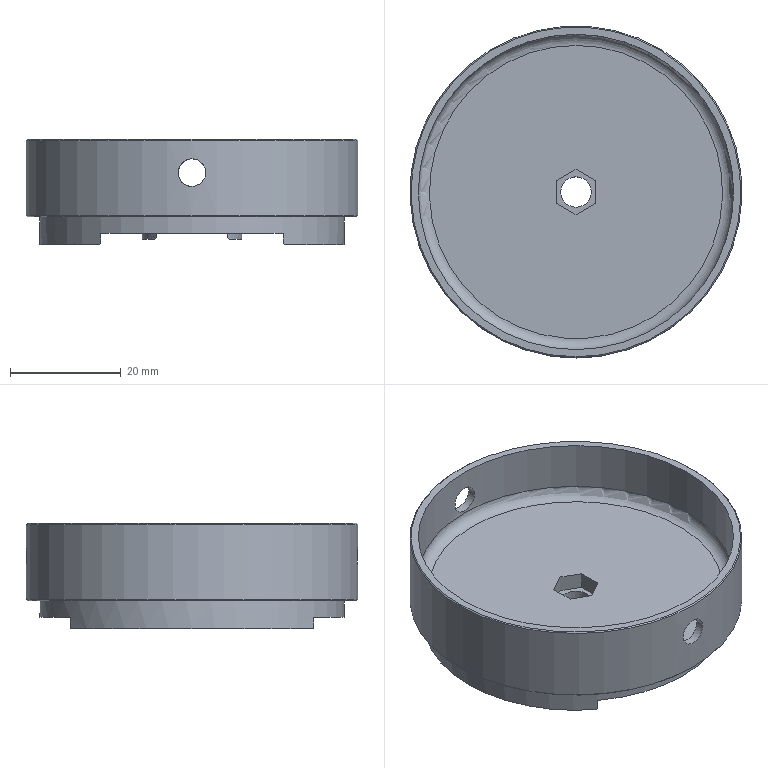NC program | NX | posted with a generic post | part box 60 x 60 x 19 mm
Lines 2835 to 4306 of 4306:
(FLOOR_WALL_1 , TOOL : D6)
N5644 T07 M6
N5646 G54
N5648 G17 G0 G90 X-2.875 Y34.477 S4500 M3
N5650 G43 Z30. H7
N5652 Z1.4
N5654 G94 G1 Z-0.1 F1000.
N5656 X-0.52 Y30.397
N5658 G3 X0. Y30.097 R0.6
N5660 G2 X16.243 Y25.337 R30.097 F1800.
N5662 G1 X13.4 Y23.916
N5664 Y-23.916
N5666 X16.243 Y-25.337
N5668 G2 X-16.243 Y-25.337 R30.097
N5670 G1 X-13.4 Y-23.916
N5672 Y23.916
N5674 X-16.243 Y25.337
N5676 G2 X0. Y30.097 R30.097
N5678 G1 Y25.897
N5680 G2 X9.21 Y24.204 R25.897
N5682 G3 X9.2 Y23.916 R4.2
N5684 G1 Y-23.916
N5686 G3 X9.21 Y-24.204 R4.2
N5688 G2 X-9.21 Y-24.204 R25.897
N5690 G3 X-9.2 Y-23.916 R4.2
N5692 G1 Y23.916
N5694 G3 X-9.21 Y24.204 R4.2
N5696 G2 X0. Y25.897 R25.897
N5698 G1 Y21.697
N5700 G2 X5. Y21.113 R21.697
N5702 G1 Y-21.113
N5704 G2 X-5. Y-21.113 R21.697
N5706 G1 Y21.113
N5708 G2 X0. Y21.697 R21.697
N5710 G1 Y17.497
N5712 G2 X0.8 Y17.479 R17.497
N5714 G1 Y-17.479
N5716 G2 X-0.8 Y-17.479 R17.497
N5718 G1 Y17.479
N5720 G2 X0. Y17.497 R17.497
N5722 G3 X0.52 Y17.797 R0.6
N5724 G1 Z1.4
N5726 G0 X-2.875 Y34.477 Z1.3
N5728 G1 Z-0.2 F1000.
N5730 X-0.52 Y30.397
N5732 G3 X0. Y30.097 R0.6
N5734 G2 X16.243 Y25.337 R30.097 F1800.
N5736 G1 X13.4 Y23.916
N5738 Y-23.916
N5740 X16.243 Y-25.337
N5742 G2 X-16.243 Y-25.337 R30.097
N5744 G1 X-13.4 Y-23.916
N5746 Y23.916
N5748 X-16.243 Y25.337
N5750 G2 X0. Y30.097 R30.097
N5752 G1 Y25.897
N5754 G2 X9.21 Y24.204 R25.897
N5756 G3 X9.2 Y23.916 R4.2
N5758 G1 Y-23.916
N5760 G3 X9.21 Y-24.204 R4.2
N5762 G2 X-9.21 Y-24.204 R25.897
N5764 G3 X-9.2 Y-23.916 R4.2
N5766 G1 Y23.916
N5768 G3 X-9.21 Y24.204 R4.2
N5770 G2 X0. Y25.897 R25.897
N5772 G1 Y21.697
N5774 G2 X5. Y21.113 R21.697
N5776 G1 Y-21.113
N5778 G2 X-5. Y-21.113 R21.697
N5780 G1 Y21.113
N5782 G2 X0. Y21.697 R21.697
N5784 G1 Y17.497
N5786 G2 X0.8 Y17.479 R17.497
N5788 G1 Y-17.479
N5790 G2 X-0.8 Y-17.479 R17.497
N5792 G1 Y17.479
N5794 G2 X0. Y17.497 R17.497
N5796 G3 X0.52 Y17.797 R0.6
N5798 G1 Z1.3
N5800 G0 X-2.875 Y34.477 Z1.2
N5802 G1 Z-0.3 F1000.
N5804 X-0.52 Y30.397
N5806 G3 X0. Y30.097 R0.6
N5808 G2 X16.243 Y25.337 R30.097 F1800.
N5810 G1 X13.4 Y23.916
N5812 Y-23.916
N5814 X16.243 Y-25.337
N5816 G2 X-16.243 Y-25.337 R30.097
N5818 G1 X-13.4 Y-23.916
N5820 Y23.916
N5822 X-16.243 Y25.337
N5824 G2 X0. Y30.097 R30.097
N5826 G1 Y25.897
N5828 G2 X9.21 Y24.204 R25.897
N5830 G3 X9.2 Y23.916 R4.2
N5832 G1 Y-23.916
N5834 G3 X9.21 Y-24.204 R4.2
N5836 G2 X-9.21 Y-24.204 R25.897
N5838 G3 X-9.2 Y-23.916 R4.2
N5840 G1 Y23.916
N5842 G3 X-9.21 Y24.204 R4.2
N5844 G2 X0. Y25.897 R25.897
N5846 G1 Y21.697
N5848 G2 X5. Y21.113 R21.697
N5850 G1 Y-21.113
N5852 G2 X-5. Y-21.113 R21.697
N5854 G1 Y21.113
N5856 G2 X0. Y21.697 R21.697
N5858 G1 Y17.497
N5860 G2 X0.8 Y17.479 R17.497
N5862 G1 Y-17.479
N5864 G2 X-0.8 Y-17.479 R17.497
N5866 G1 Y17.479
N5868 G2 X0. Y17.497 R17.497
N5870 G3 X0.52 Y17.797 R0.6
N5872 G1 Z1.2
N5874 G0 X-2.875 Y34.477 Z1.1
N5876 G1 Z-0.4 F1000.
N5878 X-0.52 Y30.397
N5880 G3 X0. Y30.097 R0.6
N5882 G2 X16.243 Y25.337 R30.097 F1800.
N5884 G1 X13.4 Y23.916
N5886 Y-23.916
N5888 X16.243 Y-25.337
N5890 G2 X-16.243 Y-25.337 R30.097
N5892 G1 X-13.4 Y-23.916
N5894 Y23.916
N5896 X-16.243 Y25.337
N5898 G2 X0. Y30.097 R30.097
N5900 G1 Y25.897
N5902 G2 X9.21 Y24.204 R25.897
N5904 G3 X9.2 Y23.916 R4.2
N5906 G1 Y-23.916
N5908 G3 X9.21 Y-24.204 R4.2
N5910 G2 X-9.21 Y-24.204 R25.897
N5912 G3 X-9.2 Y-23.916 R4.2
N5914 G1 Y23.916
N5916 G3 X-9.21 Y24.204 R4.2
N5918 G2 X0. Y25.897 R25.897
N5920 G1 Y21.697
N5922 G2 X5. Y21.113 R21.697
N5924 G1 Y-21.113
N5926 G2 X-5. Y-21.113 R21.697
N5928 G1 Y21.113
N5930 G2 X0. Y21.697 R21.697
N5932 G1 Y17.497
N5934 G2 X0.8 Y17.479 R17.497
N5936 G1 Y-17.479
N5938 G2 X-0.8 Y-17.479 R17.497
N5940 G1 Y17.479
N5942 G2 X0. Y17.497 R17.497
N5944 G3 X0.52 Y17.797 R0.6
N5946 G1 Z1.1
N5948 G0 X-2.875 Y34.477 Z1.
N5950 G1 Z-0.5 F1000.
N5952 X-0.52 Y30.397
N5954 G3 X0. Y30.097 R0.6
N5956 G2 X16.243 Y25.337 R30.097 F1800.
N5958 G1 X13.4 Y23.916
N5960 Y-23.916
N5962 X16.243 Y-25.337
N5964 G2 X-16.243 Y-25.337 R30.097
N5966 G1 X-13.4 Y-23.916
N5968 Y23.916
N5970 X-16.243 Y25.337
N5972 G2 X0. Y30.097 R30.097
N5974 G1 Y25.897
N5976 G2 X9.21 Y24.204 R25.897
N5978 G3 X9.2 Y23.916 R4.2
N5980 G1 Y-23.916
N5982 G3 X9.21 Y-24.204 R4.2
N5984 G2 X-9.21 Y-24.204 R25.897
N5986 G3 X-9.2 Y-23.916 R4.2
N5988 G1 Y23.916
N5990 G3 X-9.21 Y24.204 R4.2
N5992 G2 X0. Y25.897 R25.897
N5994 G1 Y21.697
N5996 G2 X5. Y21.113 R21.697
N5998 G1 Y-21.113
N6000 G2 X-5. Y-21.113 R21.697
N6002 G1 Y21.113
N6004 G2 X0. Y21.697 R21.697
N6006 G1 Y17.497
N6008 G2 X0.8 Y17.479 R17.497
N6010 G1 Y-17.479
N6012 G2 X-0.8 Y-17.479 R17.497
N6014 G1 Y17.479
N6016 G2 X0. Y17.497 R17.497
N6018 G3 X0.52 Y17.797 R0.6
N6020 G1 Z1.
N6022 G0 X-2.875 Y34.477 Z0.9
N6024 G1 Z-0.6 F1000.
N6026 X-0.52 Y30.397
N6028 G3 X0. Y30.097 R0.6
N6030 G2 X16.243 Y25.337 R30.097 F1800.
N6032 G1 X13.4 Y23.916
N6034 Y-23.916
N6036 X16.243 Y-25.337
N6038 G2 X-16.243 Y-25.337 R30.097
N6040 G1 X-13.4 Y-23.916
N6042 Y23.916
N6044 X-16.243 Y25.337
N6046 G2 X0. Y30.097 R30.097
N6048 G1 Y25.897
N6050 G2 X9.21 Y24.204 R25.897
N6052 G3 X9.2 Y23.916 R4.2
N6054 G1 Y-23.916
N6056 G3 X9.21 Y-24.204 R4.2
N6058 G2 X-9.21 Y-24.204 R25.897
N6060 G3 X-9.2 Y-23.916 R4.2
N6062 G1 Y23.916
N6064 G3 X-9.21 Y24.204 R4.2
N6066 G2 X0. Y25.897 R25.897
N6068 G1 Y21.697
N6070 G2 X5. Y21.113 R21.697
N6072 G1 Y-21.113
N6074 G2 X-5. Y-21.113 R21.697
N6076 G1 Y21.113
N6078 G2 X0. Y21.697 R21.697
N6080 G1 Y17.497
N6082 G2 X0.8 Y17.479 R17.497
N6084 G1 Y-17.479
N6086 G2 X-0.8 Y-17.479 R17.497
N6088 G1 Y17.479
N6090 G2 X0. Y17.497 R17.497
N6092 G3 X0.52 Y17.797 R0.6
N6094 G1 Z0.9
N6096 G0 X-2.875 Y34.477 Z0.8
N6098 G1 Z-0.7 F1000.
N6100 X-0.52 Y30.397
N6102 G3 X0. Y30.097 R0.6
N6104 G2 X16.243 Y25.337 R30.097 F1800.
N6106 G1 X13.4 Y23.916
N6108 Y-23.916
N6110 X16.243 Y-25.337
N6112 G2 X-16.243 Y-25.337 R30.097
N6114 G1 X-13.4 Y-23.916
N6116 Y23.916
N6118 X-16.243 Y25.337
N6120 G2 X0. Y30.097 R30.097
N6122 G1 Y25.897
N6124 G2 X9.21 Y24.204 R25.897
N6126 G3 X9.2 Y23.916 R4.2
N6128 G1 Y-23.916
N6130 G3 X9.21 Y-24.204 R4.2
N6132 G2 X-9.21 Y-24.204 R25.897
N6134 G3 X-9.2 Y-23.916 R4.2
N6136 G1 Y23.916
N6138 G3 X-9.21 Y24.204 R4.2
N6140 G2 X0. Y25.897 R25.897
N6142 G1 Y21.697
N6144 G2 X5. Y21.113 R21.697
N6146 G1 Y-21.113
N6148 G2 X-5. Y-21.113 R21.697
N6150 G1 Y21.113
N6152 G2 X0. Y21.697 R21.697
N6154 G1 Y17.497
N6156 G2 X0.8 Y17.479 R17.497
N6158 G1 Y-17.479
N6160 G2 X-0.8 Y-17.479 R17.497
N6162 G1 Y17.479
N6164 G2 X0. Y17.497 R17.497
N6166 G3 X0.52 Y17.797 R0.6
N6168 G1 Z0.8
N6170 G0 X-2.875 Y34.477 Z0.7
N6172 G1 Z-0.8 F1000.
N6174 X-0.52 Y30.397
N6176 G3 X0. Y30.097 R0.6
N6178 G2 X16.243 Y25.337 R30.097 F1800.
N6180 G1 X13.4 Y23.916
N6182 Y-23.916
N6184 X16.243 Y-25.337
N6186 G2 X-16.243 Y-25.337 R30.097
N6188 G1 X-13.4 Y-23.916
N6190 Y23.916
N6192 X-16.243 Y25.337
N6194 G2 X0. Y30.097 R30.097
N6196 G1 Y25.897
N6198 G2 X9.21 Y24.204 R25.897
N6200 G3 X9.2 Y23.916 R4.2
N6202 G1 Y-23.916
N6204 G3 X9.21 Y-24.204 R4.2
N6206 G2 X-9.21 Y-24.204 R25.897
N6208 G3 X-9.2 Y-23.916 R4.2
N6210 G1 Y23.916
N6212 G3 X-9.21 Y24.204 R4.2
N6214 G2 X0. Y25.897 R25.897
N6216 G1 Y21.697
N6218 G2 X5. Y21.113 R21.697
N6220 G1 Y-21.113
N6222 G2 X-5. Y-21.113 R21.697
N6224 G1 Y21.113
N6226 G2 X0. Y21.697 R21.697
N6228 G1 Y17.497
N6230 G2 X0.8 Y17.479 R17.497
N6232 G1 Y-17.479
N6234 G2 X-0.8 Y-17.479 R17.497
N6236 G1 Y17.479
N6238 G2 X0. Y17.497 R17.497
N6240 G3 X0.52 Y17.797 R0.6
N6242 G1 Z0.7
N6244 G0 X-2.875 Y34.477 Z0.6
N6246 G1 Z-0.9 F1000.
N6248 X-0.52 Y30.397
N6250 G3 X0. Y30.097 R0.6
N6252 G2 X16.243 Y25.337 R30.097 F1800.
N6254 G1 X13.4 Y23.916
N6256 Y-23.916
N6258 X16.243 Y-25.337
N6260 G2 X-16.243 Y-25.337 R30.097
N6262 G1 X-13.4 Y-23.916
N6264 Y23.916
N6266 X-16.243 Y25.337
N6268 G2 X0. Y30.097 R30.097
N6270 G1 Y25.897
N6272 G2 X9.21 Y24.204 R25.897
N6274 G3 X9.2 Y23.916 R4.2
N6276 G1 Y-23.916
N6278 G3 X9.21 Y-24.204 R4.2
N6280 G2 X-9.21 Y-24.204 R25.897
N6282 G3 X-9.2 Y-23.916 R4.2
N6284 G1 Y23.916
N6286 G3 X-9.21 Y24.204 R4.2
N6288 G2 X0. Y25.897 R25.897
N6290 G1 Y21.697
N6292 G2 X5. Y21.113 R21.697
N6294 G1 Y-21.113
N6296 G2 X-5. Y-21.113 R21.697
N6298 G1 Y21.113
N6300 G2 X0. Y21.697 R21.697
N6302 G1 Y17.497
N6304 G2 X0.8 Y17.479 R17.497
N6306 G1 Y-17.479
N6308 G2 X-0.8 Y-17.479 R17.497
N6310 G1 Y17.479
N6312 G2 X0. Y17.497 R17.497
N6314 G3 X0.52 Y17.797 R0.6
N6316 G1 Z0.6
N6318 G0 Z30.
N6320 X-2.875 Y34.477
N6322 Z0.4
N6324 G1 Z-1.1 F1000.
N6326 X-0.52 Y30.397
N6328 G3 X0. Y30.097 R0.6
N6330 G2 X16.243 Y25.337 R30.097 F1800.
N6332 G1 X13.4 Y23.916
N6334 Y-23.916
N6336 X16.243 Y-25.337
N6338 G2 X-16.243 Y-25.337 R30.097
N6340 G1 X-13.4 Y-23.916
N6342 Y23.916
N6344 X-16.243 Y25.337
N6346 G2 X0. Y30.097 R30.097
N6348 G1 Y25.897
N6350 G2 X9.21 Y24.204 R25.897
N6352 G3 X9.2 Y23.916 R4.2
N6354 G1 Y9.102
N6356 X7.896 Y10.464
N6358 G3 X6.976 Y10.662 R0.84
N6360 G1 X3.087 Y9.1
N6362 G3 X2.56 Y8.321 R0.84
N6364 G1 Y-8.321
N6366 G3 X3.087 Y-9.1 R0.84
N6368 G1 X6.976 Y-10.662
N6370 G3 X7.896 Y-10.464 R0.84
N6372 G1 X9.2 Y-9.102
N6374 X8.593 Y-8.521
N6376 X7.289 Y-9.883
N6378 X3.4 Y-8.321
N6380 Y8.321
N6382 X7.289 Y9.883
N6384 X8.739 Y8.369
N6386 G2 X8.739 Y-8.369 R12.1
N6388 G1 X8.593 Y-8.521
N6390 X9.2 Y-9.102
N6392 Y-23.916
N6394 G3 X9.21 Y-24.204 R4.2
N6396 G2 X-9.21 Y-24.204 R25.897
N6398 G3 X-9.2 Y-23.916 R4.2
N6400 G1 Y-9.102
N6402 X-7.896 Y-10.464
N6404 G3 X-6.976 Y-10.662 R0.84
N6406 G1 X-3.087 Y-9.1
N6408 G3 X-2.833 Y-8.941 R0.84
N6410 G1 X0. Y-12.041
N6412 G3 X1.565 Y-13.015 R5.04
N6414 G1 X5. Y-14.394
N6416 Y-21.113
N6418 G2 X-5. Y-21.113 R21.697
N6420 G1 Y-14.394
N6422 X-1.522 Y-12.998
N6424 G3 X0. Y-12.041 R5.04
N6426 G1 Y-16.912
N6428 X0.8 Y-17.234
N6430 Y-17.479
N6432 G2 X-0.8 Y-17.479 R17.497
N6434 G1 Y-17.234
N6436 X0. Y-16.912
N6438 Y-12.041
N6440 X-2.833 Y-8.941
N6442 G3 X-2.56 Y-8.321 R0.84
N6444 G1 Y8.321
N6446 G3 X-3.087 Y9.1 R0.84
N6448 G1 X-6.976 Y10.662
N6450 G3 X-7.896 Y10.464 R0.84
N6452 G1 X-9.2 Y9.102
N6454 X-8.593 Y8.521
N6456 X-7.289 Y9.883
N6458 X-3.4 Y8.321
N6460 Y-8.321
N6462 X-7.289 Y-9.883
N6464 X-8.739 Y-8.369
N6466 G2 X-8.739 Y8.369 R12.1
N6468 G1 X-8.593 Y8.521
N6470 X-9.2 Y9.102
N6472 Y23.916
N6474 G3 X-9.21 Y24.204 R4.2
N6476 G2 X0. Y25.897 R25.897
N6478 G1 Y21.697
N6480 G2 X5. Y21.113 R21.697
N6482 G1 Y14.394
N6484 X1.522 Y12.998
N6486 G3 X0. Y12.041 R5.04
N6488 X-1.565 Y13.015 R5.04
N6490 G1 X-5. Y14.394
N6492 Y21.113
N6494 G2 X0. Y21.697 R21.697
N6496 G1 Y17.497
N6498 G2 X0.8 Y17.479 R17.497
N6500 G1 Y17.234
N6502 X0. Y16.912
N6504 X-0.8 Y17.234
N6506 Y17.479
N6508 G2 X0. Y17.497 R17.497
N6510 G3 X0.52 Y17.797 R0.6
N6512 G1 Z0.4
N6514 G0 X-2.875 Y34.477 Z0.3
N6516 G1 Z-1.2 F1000.
N6518 X-0.52 Y30.397
N6520 G3 X0. Y30.097 R0.6
N6522 G2 X16.243 Y25.337 R30.097 F1800.
N6524 G1 X13.4 Y23.916
N6526 Y-23.916
N6528 X16.243 Y-25.337
N6530 G2 X-16.243 Y-25.337 R30.097
N6532 G1 X-13.4 Y-23.916
N6534 Y23.916
N6536 X-16.243 Y25.337
N6538 G2 X0. Y30.097 R30.097
N6540 G1 Y25.897
N6542 G2 X9.21 Y24.204 R25.897
N6544 G3 X9.2 Y23.916 R4.2
N6546 G1 Y9.102
N6548 X7.896 Y10.464
N6550 G3 X6.976 Y10.662 R0.84
N6552 G1 X3.087 Y9.1
N6554 G3 X2.56 Y8.321 R0.84
N6556 G1 Y-8.321
N6558 G3 X3.087 Y-9.1 R0.84
N6560 G1 X6.976 Y-10.662
N6562 G3 X7.896 Y-10.464 R0.84
N6564 G1 X9.2 Y-9.102
N6566 X8.593 Y-8.521
N6568 X7.289 Y-9.883
N6570 X3.4 Y-8.321
N6572 Y8.321
N6574 X7.289 Y9.883
N6576 X8.739 Y8.369
N6578 G2 X8.739 Y-8.369 R12.1
N6580 G1 X8.593 Y-8.521
N6582 X9.2 Y-9.102
N6584 Y-23.916
N6586 G3 X9.21 Y-24.204 R4.2
N6588 G2 X-9.21 Y-24.204 R25.897
N6590 G3 X-9.2 Y-23.916 R4.2
N6592 G1 Y-9.102
N6594 X-7.896 Y-10.464
N6596 G3 X-6.976 Y-10.662 R0.84
N6598 G1 X-3.087 Y-9.1
N6600 G3 X-2.833 Y-8.941 R0.84
N6602 G1 X0. Y-12.041
N6604 G3 X1.565 Y-13.015 R5.04
N6606 G1 X5. Y-14.394
N6608 Y-21.113
N6610 G2 X-5. Y-21.113 R21.697
N6612 G1 Y-14.394
N6614 X-1.522 Y-12.998
N6616 G3 X0. Y-12.041 R5.04
N6618 G1 Y-16.912
N6620 X0.8 Y-17.234
N6622 Y-17.479
N6624 G2 X-0.8 Y-17.479 R17.497
N6626 G1 Y-17.234
N6628 X0. Y-16.912
N6630 Y-12.041
N6632 X-2.833 Y-8.941
N6634 G3 X-2.56 Y-8.321 R0.84
N6636 G1 Y8.321
N6638 G3 X-3.087 Y9.1 R0.84
N6640 G1 X-6.976 Y10.662
N6642 G3 X-7.896 Y10.464 R0.84
N6644 G1 X-9.2 Y9.102
N6646 X-8.593 Y8.521
N6648 X-7.289 Y9.883
N6650 X-3.4 Y8.321
N6652 Y-8.321
N6654 X-7.289 Y-9.883
N6656 X-8.739 Y-8.369
N6658 G2 X-8.739 Y8.369 R12.1
N6660 G1 X-8.593 Y8.521
N6662 X-9.2 Y9.102
N6664 Y23.916
N6666 G3 X-9.21 Y24.204 R4.2
N6668 G2 X0. Y25.897 R25.897
N6670 G1 Y21.697
N6672 G2 X5. Y21.113 R21.697
N6674 G1 Y14.394
N6676 X1.522 Y12.998
N6678 G3 X0. Y12.041 R5.04
N6680 X-1.565 Y13.015 R5.04
N6682 G1 X-5. Y14.394
N6684 Y21.113
N6686 G2 X0. Y21.697 R21.697
N6688 G1 Y17.497
N6690 G2 X0.8 Y17.479 R17.497
N6692 G1 Y17.234
N6694 X0. Y16.912
N6696 X-0.8 Y17.234
N6698 Y17.479
N6700 G2 X0. Y17.497 R17.497
N6702 G3 X0.52 Y17.797 R0.6
N6704 G1 Z0.3
N6706 G0 X-2.875 Y34.477 Z0.2
N6708 G1 Z-1.3 F1000.
N6710 X-0.52 Y30.397
N6712 G3 X0. Y30.097 R0.6
N6714 G2 X16.243 Y25.337 R30.097 F1800.
N6716 G1 X13.4 Y23.916
N6718 Y-23.916
N6720 X16.243 Y-25.337
N6722 G2 X-16.243 Y-25.337 R30.097
N6724 G1 X-13.4 Y-23.916
N6726 Y23.916
N6728 X-16.243 Y25.337
N6730 G2 X0. Y30.097 R30.097
N6732 G1 Y25.897
N6734 G2 X9.21 Y24.204 R25.897
N6736 G3 X9.2 Y23.916 R4.2
N6738 G1 Y9.102
N6740 X7.896 Y10.464
N6742 G3 X6.976 Y10.662 R0.84
N6744 G1 X3.087 Y9.1
N6746 G3 X2.56 Y8.321 R0.84
N6748 G1 Y-8.321
N6750 G3 X3.087 Y-9.1 R0.84
N6752 G1 X6.976 Y-10.662
N6754 G3 X7.896 Y-10.464 R0.84
N6756 G1 X9.2 Y-9.102
N6758 X8.593 Y-8.521
N6760 X7.289 Y-9.883
N6762 X3.4 Y-8.321
N6764 Y8.321
N6766 X7.289 Y9.883
N6768 X8.739 Y8.369
N6770 G2 X8.739 Y-8.369 R12.1
N6772 G1 X8.593 Y-8.521
N6774 X9.2 Y-9.102
N6776 Y-23.916
N6778 G3 X9.21 Y-24.204 R4.2
N6780 G2 X-9.21 Y-24.204 R25.897
N6782 G3 X-9.2 Y-23.916 R4.2
N6784 G1 Y-9.102
N6786 X-7.896 Y-10.464
N6788 G3 X-6.976 Y-10.662 R0.84
N6790 G1 X-3.087 Y-9.1
N6792 G3 X-2.833 Y-8.941 R0.84
N6794 G1 X0. Y-12.041
N6796 G3 X1.565 Y-13.015 R5.04
N6798 G1 X5. Y-14.394
N6800 Y-21.113
N6802 G2 X-5. Y-21.113 R21.697
N6804 G1 Y-14.394
N6806 X-1.522 Y-12.998
N6808 G3 X0. Y-12.041 R5.04
N6810 G1 Y-16.912
N6812 X0.8 Y-17.234
N6814 Y-17.479
N6816 G2 X-0.8 Y-17.479 R17.497
N6818 G1 Y-17.234
N6820 X0. Y-16.912
N6822 Y-12.041
N6824 X-2.833 Y-8.941
N6826 G3 X-2.56 Y-8.321 R0.84
N6828 G1 Y8.321
N6830 G3 X-3.087 Y9.1 R0.84
N6832 G1 X-6.976 Y10.662
N6834 G3 X-7.896 Y10.464 R0.84
N6836 G1 X-9.2 Y9.102
N6838 X-8.593 Y8.521
N6840 X-7.289 Y9.883
N6842 X-3.4 Y8.321
N6844 Y-8.321
N6846 X-7.289 Y-9.883
N6848 X-8.739 Y-8.369
N6850 G2 X-8.739 Y8.369 R12.1
N6852 G1 X-8.593 Y8.521
N6854 X-9.2 Y9.102
N6856 Y23.916
N6858 G3 X-9.21 Y24.204 R4.2
N6860 G2 X0. Y25.897 R25.897
N6862 G1 Y21.697
N6864 G2 X5. Y21.113 R21.697
N6866 G1 Y14.394
N6868 X1.522 Y12.998
N6870 G3 X0. Y12.041 R5.04
N6872 X-1.565 Y13.015 R5.04
N6874 G1 X-5. Y14.394
N6876 Y21.113
N6878 G2 X0. Y21.697 R21.697
N6880 G1 Y17.497
N6882 G2 X0.8 Y17.479 R17.497
N6884 G1 Y17.234
N6886 X0. Y16.912
N6888 X-0.8 Y17.234
N6890 Y17.479
N6892 G2 X0. Y17.497 R17.497
N6894 G3 X0.52 Y17.797 R0.6
N6896 G1 Z0.2
N6898 G0 X-2.875 Y34.477 Z0.1
N6900 G1 Z-1.4 F1000.
N6902 X-0.52 Y30.397
N6904 G3 X0. Y30.097 R0.6
N6906 G2 X16.243 Y25.337 R30.097 F1800.
N6908 G1 X13.4 Y23.916
N6910 Y-23.916
N6912 X16.243 Y-25.337
N6914 G2 X-16.243 Y-25.337 R30.097
N6916 G1 X-13.4 Y-23.916
N6918 Y23.916
N6920 X-16.243 Y25.337
N6922 G2 X0. Y30.097 R30.097
N6924 G1 Y25.897
N6926 G2 X9.21 Y24.204 R25.897
N6928 G3 X9.2 Y23.916 R4.2
N6930 G1 Y9.102
N6932 X7.896 Y10.464
N6934 G3 X6.976 Y10.662 R0.84
N6936 G1 X3.087 Y9.1
N6938 G3 X2.56 Y8.321 R0.84
N6940 G1 Y-8.321
N6942 G3 X3.087 Y-9.1 R0.84
N6944 G1 X6.976 Y-10.662
N6946 G3 X7.896 Y-10.464 R0.84
N6948 G1 X9.2 Y-9.102
N6950 X8.593 Y-8.521
N6952 X7.289 Y-9.883
N6954 X3.4 Y-8.321
N6956 Y8.321
N6958 X7.289 Y9.883
N6960 X8.739 Y8.369
N6962 G2 X8.739 Y-8.369 R12.1
N6964 G1 X8.593 Y-8.521
N6966 X9.2 Y-9.102
N6968 Y-23.916
N6970 G3 X9.21 Y-24.204 R4.2
N6972 G2 X-9.21 Y-24.204 R25.897
N6974 G3 X-9.2 Y-23.916 R4.2
N6976 G1 Y-9.102
N6978 X-7.896 Y-10.464
N6980 G3 X-6.976 Y-10.662 R0.84
N6982 G1 X-3.087 Y-9.1
N6984 G3 X-2.833 Y-8.941 R0.84
N6986 G1 X0. Y-12.041
N6988 G3 X1.565 Y-13.015 R5.04
N6990 G1 X5. Y-14.394
N6992 Y-21.113
N6994 G2 X-5. Y-21.113 R21.697
N6996 G1 Y-14.394
N6998 X-1.522 Y-12.998
N7000 G3 X0. Y-12.041 R5.04
N7002 G1 Y-16.912
N7004 X0.8 Y-17.234
N7006 Y-17.479
N7008 G2 X-0.8 Y-17.479 R17.497
N7010 G1 Y-17.234
N7012 X0. Y-16.912
N7014 Y-12.041
N7016 X-2.833 Y-8.941
N7018 G3 X-2.56 Y-8.321 R0.84
N7020 G1 Y8.321
N7022 G3 X-3.087 Y9.1 R0.84
N7024 G1 X-6.976 Y10.662
N7026 G3 X-7.896 Y10.464 R0.84
N7028 G1 X-9.2 Y9.102
N7030 X-8.593 Y8.521
N7032 X-7.289 Y9.883
N7034 X-3.4 Y8.321
N7036 Y-8.321
N7038 X-7.289 Y-9.883
N7040 X-8.739 Y-8.369
N7042 G2 X-8.739 Y8.369 R12.1
N7044 G1 X-8.593 Y8.521
N7046 X-9.2 Y9.102
N7048 Y23.916
N7050 G3 X-9.21 Y24.204 R4.2
N7052 G2 X0. Y25.897 R25.897
N7054 G1 Y21.697
N7056 G2 X5. Y21.113 R21.697
N7058 G1 Y14.394
N7060 X1.522 Y12.998
N7062 G3 X0. Y12.041 R5.04
N7064 X-1.565 Y13.015 R5.04
N7066 G1 X-5. Y14.394
N7068 Y21.113
N7070 G2 X0. Y21.697 R21.697
N7072 G1 Y17.497
N7074 G2 X0.8 Y17.479 R17.497
N7076 G1 Y17.234
N7078 X0. Y16.912
N7080 X-0.8 Y17.234
N7082 Y17.479
N7084 G2 X0. Y17.497 R17.497
N7086 G3 X0.52 Y17.797 R0.6
N7088 G1 Z0.1
N7090 G0 X-2.875 Y34.477 Z0.
N7092 G1 Z-1.5 F1000.
N7094 X-0.52 Y30.397
N7096 G3 X0. Y30.097 R0.6
N7098 G2 X16.243 Y25.337 R30.097 F1800.
N7100 G1 X13.4 Y23.916
N7102 Y-23.916
N7104 X16.243 Y-25.337
N7106 G2 X-16.243 Y-25.337 R30.097
N7108 G1 X-13.4 Y-23.916
N7110 Y23.916
N7112 X-16.243 Y25.337
N7114 G2 X0. Y30.097 R30.097
N7116 G1 Y25.897
N7118 G2 X9.21 Y24.204 R25.897
N7120 G3 X9.2 Y23.916 R4.2
N7122 G1 Y9.102
N7124 X7.896 Y10.464
N7126 G3 X6.976 Y10.662 R0.84
N7128 G1 X3.087 Y9.1
N7130 G3 X2.56 Y8.321 R0.84
N7132 G1 Y-8.321
N7134 G3 X3.087 Y-9.1 R0.84
N7136 G1 X6.976 Y-10.662
N7138 G3 X7.896 Y-10.464 R0.84
N7140 G1 X9.2 Y-9.102
N7142 X8.593 Y-8.521
N7144 X7.289 Y-9.883
N7146 X3.4 Y-8.321
N7148 Y8.321
N7150 X7.289 Y9.883
N7152 X8.739 Y8.369
N7154 G2 X8.739 Y-8.369 R12.1
N7156 G1 X8.593 Y-8.521
N7158 X9.2 Y-9.102
N7160 Y-23.916
N7162 G3 X9.21 Y-24.204 R4.2
N7164 G2 X-9.21 Y-24.204 R25.897
N7166 G3 X-9.2 Y-23.916 R4.2
N7168 G1 Y-9.102
N7170 X-7.896 Y-10.464
N7172 G3 X-6.976 Y-10.662 R0.84
N7174 G1 X-3.087 Y-9.1
N7176 G3 X-2.833 Y-8.941 R0.84
N7178 G1 X0. Y-12.041
N7180 G3 X1.565 Y-13.015 R5.04
N7182 G1 X5. Y-14.394
N7184 Y-21.113
N7186 G2 X-5. Y-21.113 R21.697
N7188 G1 Y-14.394
N7190 X-1.522 Y-12.998
N7192 G3 X0. Y-12.041 R5.04
N7194 G1 Y-16.912
N7196 X0.8 Y-17.234
N7198 Y-17.479
N7200 G2 X-0.8 Y-17.479 R17.497
N7202 G1 Y-17.234
N7204 X0. Y-16.912
N7206 Y-12.041
N7208 X-2.833 Y-8.941
N7210 G3 X-2.56 Y-8.321 R0.84
N7212 G1 Y8.321
N7214 G3 X-3.087 Y9.1 R0.84
N7216 G1 X-6.976 Y10.662
N7218 G3 X-7.896 Y10.464 R0.84
N7220 G1 X-9.2 Y9.102
N7222 X-8.593 Y8.521
N7224 X-7.289 Y9.883
N7226 X-3.4 Y8.321
N7228 Y-8.321
N7230 X-7.289 Y-9.883
N7232 X-8.739 Y-8.369
N7234 G2 X-8.739 Y8.369 R12.1
N7236 G1 X-8.593 Y8.521
N7238 X-9.2 Y9.102
N7240 Y23.916
N7242 G3 X-9.21 Y24.204 R4.2
N7244 G2 X0. Y25.897 R25.897
N7246 G1 Y21.697
N7248 G2 X5. Y21.113 R21.697
N7250 G1 Y14.394
N7252 X1.522 Y12.998
N7254 G3 X0. Y12.041 R5.04
N7256 X-1.565 Y13.015 R5.04
N7258 G1 X-5. Y14.394
N7260 Y21.113
N7262 G2 X0. Y21.697 R21.697
N7264 G1 Y17.497
N7266 G2 X0.8 Y17.479 R17.497
N7268 G1 Y17.234
N7270 X0. Y16.912
N7272 X-0.8 Y17.234
N7274 Y17.479
N7276 G2 X0. Y17.497 R17.497
N7278 G3 X0.52 Y17.797 R0.6
N7280 G1 Z0.
N7282 G0 X-2.875 Y34.477 Z-0.1
N7284 G1 Z-1.6 F1000.
N7286 X-0.52 Y30.397
N7288 G3 X0. Y30.097 R0.6
N7290 G2 X16.243 Y25.337 R30.097 F1800.
N7292 G1 X13.4 Y23.916
N7294 Y-23.916
N7296 X16.243 Y-25.337
N7298 G2 X-16.243 Y-25.337 R30.097
N7300 G1 X-13.4 Y-23.916
N7302 Y23.916
N7304 X-16.243 Y25.337
N7306 G2 X0. Y30.097 R30.097
N7308 G1 Y25.897
N7310 G2 X9.21 Y24.204 R25.897
N7312 G3 X9.2 Y23.916 R4.2
N7314 G1 Y9.102
N7316 X7.896 Y10.464
N7318 G3 X6.976 Y10.662 R0.84
N7320 G1 X3.087 Y9.1
N7322 G3 X2.56 Y8.321 R0.84
N7324 G1 Y-8.321
N7326 G3 X3.087 Y-9.1 R0.84
N7328 G1 X6.976 Y-10.662
N7330 G3 X7.896 Y-10.464 R0.84
N7332 G1 X9.2 Y-9.102
N7334 X8.593 Y-8.521
N7336 X7.289 Y-9.883
N7338 X3.4 Y-8.321
N7340 Y8.321
N7342 X7.289 Y9.883
N7344 X8.739 Y8.369
N7346 G2 X8.739 Y-8.369 R12.1
N7348 G1 X8.593 Y-8.521
N7350 X9.2 Y-9.102
N7352 Y-23.916
N7354 G3 X9.21 Y-24.204 R4.2
N7356 G2 X-9.21 Y-24.204 R25.897
N7358 G3 X-9.2 Y-23.916 R4.2
N7360 G1 Y-9.102
N7362 X-7.896 Y-10.464
N7364 G3 X-6.976 Y-10.662 R0.84
N7366 G1 X-3.087 Y-9.1
N7368 G3 X-2.833 Y-8.941 R0.84
N7370 G1 X0. Y-12.041
N7372 G3 X1.565 Y-13.015 R5.04
N7374 G1 X5. Y-14.394
N7376 Y-21.113
N7378 G2 X-5. Y-21.113 R21.697
N7380 G1 Y-14.394
N7382 X-1.522 Y-12.998
N7384 G3 X0. Y-12.041 R5.04
N7386 G1 Y-16.912
N7388 X0.8 Y-17.234
N7390 Y-17.479
N7392 G2 X-0.8 Y-17.479 R17.497
N7394 G1 Y-17.234
N7396 X0. Y-16.912
N7398 Y-12.041
N7400 X-2.833 Y-8.941
N7402 G3 X-2.56 Y-8.321 R0.84
N7404 G1 Y8.321
N7406 G3 X-3.087 Y9.1 R0.84
N7408 G1 X-6.976 Y10.662
N7410 G3 X-7.896 Y10.464 R0.84
N7412 G1 X-9.2 Y9.102
N7414 X-8.593 Y8.521
N7416 X-7.289 Y9.883
N7418 X-3.4 Y8.321
N7420 Y-8.321
N7422 X-7.289 Y-9.883
N7424 X-8.739 Y-8.369
N7426 G2 X-8.739 Y8.369 R12.1
N7428 G1 X-8.593 Y8.521
N7430 X-9.2 Y9.102
N7432 Y23.916
N7434 G3 X-9.21 Y24.204 R4.2
N7436 G2 X0. Y25.897 R25.897
N7438 G1 Y21.697
N7440 G2 X5. Y21.113 R21.697
N7442 G1 Y14.394
N7444 X1.522 Y12.998
N7446 G3 X0. Y12.041 R5.04
N7448 X-1.565 Y13.015 R5.04
N7450 G1 X-5. Y14.394
N7452 Y21.113
N7454 G2 X0. Y21.697 R21.697
N7456 G1 Y17.497
N7458 G2 X0.8 Y17.479 R17.497
N7460 G1 Y17.234
N7462 X0. Y16.912
N7464 X-0.8 Y17.234
N7466 Y17.479
N7468 G2 X0. Y17.497 R17.497
N7470 G3 X0.52 Y17.797 R0.6
N7472 G1 Z-0.1
N7474 G0 X-2.875 Y34.477 Z-0.2
N7476 G1 Z-1.7 F1000.
N7478 X-0.52 Y30.397
N7480 G3 X0. Y30.097 R0.6
N7482 G2 X16.243 Y25.337 R30.097 F1800.
N7484 G1 X13.4 Y23.916
N7486 Y-23.916
N7488 X16.243 Y-25.337
N7490 G2 X-16.243 Y-25.337 R30.097
N7492 G1 X-13.4 Y-23.916
N7494 Y23.916
N7496 X-16.243 Y25.337
N7498 G2 X0. Y30.097 R30.097
N7500 G1 Y25.897
N7502 G2 X9.21 Y24.204 R25.897
N7504 G3 X9.2 Y23.916 R4.2
N7506 G1 Y9.102
N7508 X7.896 Y10.464
N7510 G3 X6.976 Y10.662 R0.84
N7512 G1 X3.087 Y9.1
N7514 G3 X2.56 Y8.321 R0.84
N7516 G1 Y-8.321
N7518 G3 X3.087 Y-9.1 R0.84
N7520 G1 X6.976 Y-10.662
N7522 G3 X7.896 Y-10.464 R0.84
N7524 G1 X9.2 Y-9.102
N7526 X8.593 Y-8.521
N7528 X7.289 Y-9.883
N7530 X3.4 Y-8.321
N7532 Y8.321
N7534 X7.289 Y9.883
N7536 X8.739 Y8.369
N7538 G2 X8.739 Y-8.369 R12.1
N7540 G1 X8.593 Y-8.521
N7542 X9.2 Y-9.102
N7544 Y-23.916
N7546 G3 X9.21 Y-24.204 R4.2
N7548 G2 X-9.21 Y-24.204 R25.897
N7550 G3 X-9.2 Y-23.916 R4.2
N7552 G1 Y-9.102
N7554 X-7.896 Y-10.464
N7556 G3 X-6.976 Y-10.662 R0.84
N7558 G1 X-3.087 Y-9.1
N7560 G3 X-2.833 Y-8.941 R0.84
N7562 G1 X0. Y-12.041
N7564 G3 X1.565 Y-13.015 R5.04
N7566 G1 X5. Y-14.394
N7568 Y-21.113
N7570 G2 X-5. Y-21.113 R21.697
N7572 G1 Y-14.394
N7574 X-1.522 Y-12.998
N7576 G3 X0. Y-12.041 R5.04
N7578 G1 Y-16.912
N7580 X0.8 Y-17.234
N7582 Y-17.479
N7584 G2 X-0.8 Y-17.479 R17.497
N7586 G1 Y-17.234
N7588 X0. Y-16.912
N7590 Y-12.041
N7592 X-2.833 Y-8.941
N7594 G3 X-2.56 Y-8.321 R0.84
N7596 G1 Y8.321
N7598 G3 X-3.087 Y9.1 R0.84
N7600 G1 X-6.976 Y10.662
N7602 G3 X-7.896 Y10.464 R0.84
N7604 G1 X-9.2 Y9.102
N7606 X-8.593 Y8.521
N7608 X-7.289 Y9.883
N7610 X-3.4 Y8.321
N7612 Y-8.321
N7614 X-7.289 Y-9.883
N7616 X-8.739 Y-8.369
N7618 G2 X-8.739 Y8.369 R12.1
N7620 G1 X-8.593 Y8.521
N7622 X-9.2 Y9.102
N7624 Y23.916
N7626 G3 X-9.21 Y24.204 R4.2
N7628 G2 X0. Y25.897 R25.897
N7630 G1 Y21.697
N7632 G2 X5. Y21.113 R21.697
N7634 G1 Y14.394
N7636 X1.522 Y12.998
N7638 G3 X0. Y12.041 R5.04
N7640 X-1.565 Y13.015 R5.04
N7642 G1 X-5. Y14.394
N7644 Y21.113
N7646 G2 X0. Y21.697 R21.697
N7648 G1 Y17.497
N7650 G2 X0.8 Y17.479 R17.497
N7652 G1 Y17.234
N7654 X0. Y16.912
N7656 X-0.8 Y17.234
N7658 Y17.479
N7660 G2 X0. Y17.497 R17.497
N7662 G3 X0.52 Y17.797 R0.6
N7664 G1 Z-0.2
N7666 G0 X-2.875 Y34.477 Z-0.3
N7668 G1 Z-1.8 F1000.
N7670 X-0.52 Y30.397
N7672 G3 X0. Y30.097 R0.6
N7674 G2 X16.243 Y25.337 R30.097 F1800.
N7676 G1 X13.4 Y23.916
N7678 Y-23.916
N7680 X16.243 Y-25.337
N7682 G2 X-16.243 Y-25.337 R30.097
N7684 G1 X-13.4 Y-23.916
N7686 Y23.916
N7688 X-16.243 Y25.337
N7690 G2 X0. Y30.097 R30.097
N7692 G1 Y25.897
N7694 G2 X9.21 Y24.204 R25.897
N7696 G3 X9.2 Y23.916 R4.2
N7698 G1 Y9.102
N7700 X7.896 Y10.464
N7702 G3 X6.976 Y10.662 R0.84
N7704 G1 X3.087 Y9.1
N7706 G3 X2.56 Y8.321 R0.84
N7708 G1 Y-8.321
N7710 G3 X3.087 Y-9.1 R0.84
N7712 G1 X6.976 Y-10.662
N7714 G3 X7.896 Y-10.464 R0.84
N7716 G1 X9.2 Y-9.102
N7718 X8.593 Y-8.521
N7720 X7.289 Y-9.883
N7722 X3.4 Y-8.321
N7724 Y8.321
N7726 X7.289 Y9.883
N7728 X8.739 Y8.369
N7730 G2 X8.739 Y-8.369 R12.1
N7732 G1 X8.593 Y-8.521
N7734 X9.2 Y-9.102
N7736 Y-23.916
N7738 G3 X9.21 Y-24.204 R4.2
N7740 G2 X-9.21 Y-24.204 R25.897
N7742 G3 X-9.2 Y-23.916 R4.2
N7744 G1 Y-9.102
N7746 X-7.896 Y-10.464
N7748 G3 X-6.976 Y-10.662 R0.84
N7750 G1 X-3.087 Y-9.1
N7752 G3 X-2.833 Y-8.941 R0.84
N7754 G1 X0. Y-12.041
N7756 G3 X1.565 Y-13.015 R5.04
N7758 G1 X5. Y-14.394
N7760 Y-21.113
N7762 G2 X-5. Y-21.113 R21.697
N7764 G1 Y-14.394
N7766 X-1.522 Y-12.998
N7768 G3 X0. Y-12.041 R5.04
N7770 G1 Y-16.912
N7772 X0.8 Y-17.234
N7774 Y-17.479
N7776 G2 X-0.8 Y-17.479 R17.497
N7778 G1 Y-17.234
N7780 X0. Y-16.912
N7782 Y-12.041
N7784 X-2.833 Y-8.941
N7786 G3 X-2.56 Y-8.321 R0.84
N7788 G1 Y8.321
N7790 G3 X-3.087 Y9.1 R0.84
N7792 G1 X-6.976 Y10.662
N7794 G3 X-7.896 Y10.464 R0.84
N7796 G1 X-9.2 Y9.102
N7798 X-8.593 Y8.521
N7800 X-7.289 Y9.883
N7802 X-3.4 Y8.321
N7804 Y-8.321
N7806 X-7.289 Y-9.883
N7808 X-8.739 Y-8.369
N7810 G2 X-8.739 Y8.369 R12.1
N7812 G1 X-8.593 Y8.521
N7814 X-9.2 Y9.102
N7816 Y23.916
N7818 G3 X-9.21 Y24.204 R4.2
N7820 G2 X0. Y25.897 R25.897
N7822 G1 Y21.697
N7824 G2 X5. Y21.113 R21.697
N7826 G1 Y14.394
N7828 X1.522 Y12.998
N7830 G3 X0. Y12.041 R5.04
N7832 X-1.565 Y13.015 R5.04
N7834 G1 X-5. Y14.394
N7836 Y21.113
N7838 G2 X0. Y21.697 R21.697
N7840 G1 Y17.497
N7842 G2 X0.8 Y17.479 R17.497
N7844 G1 Y17.234
N7846 X0. Y16.912
N7848 X-0.8 Y17.234
N7850 Y17.479
N7852 G2 X0. Y17.497 R17.497
N7854 G3 X0.52 Y17.797 R0.6
N7856 G1 Z-0.3
N7858 G0 X-2.875 Y34.477 Z-0.4
N7860 G1 Z-1.9 F1000.
N7862 X-0.52 Y30.397
N7864 G3 X0. Y30.097 R0.6
N7866 G2 X16.243 Y25.337 R30.097 F1800.
N7868 G1 X13.4 Y23.916
N7870 Y-23.916
N7872 X16.243 Y-25.337
N7874 G2 X-16.243 Y-25.337 R30.097
N7876 G1 X-13.4 Y-23.916
N7878 Y23.916
N7880 X-16.243 Y25.337
N7882 G2 X0. Y30.097 R30.097
N7884 G1 Y25.897
N7886 G2 X9.21 Y24.204 R25.897
N7888 G3 X9.2 Y23.916 R4.2
N7890 G1 Y9.102
N7892 X7.896 Y10.464
N7894 G3 X6.976 Y10.662 R0.84
N7896 G1 X3.087 Y9.1
N7898 G3 X2.56 Y8.321 R0.84
N7900 G1 Y-8.321
N7902 G3 X3.087 Y-9.1 R0.84
N7904 G1 X6.976 Y-10.662
N7906 G3 X7.896 Y-10.464 R0.84
N7908 G1 X9.2 Y-9.102
N7910 X8.593 Y-8.521
N7912 X7.289 Y-9.883
N7914 X3.4 Y-8.321
N7916 Y8.321
N7918 X7.289 Y9.883
N7920 X8.739 Y8.369
N7922 G2 X8.739 Y-8.369 R12.1
N7924 G1 X8.593 Y-8.521
N7926 X9.2 Y-9.102
N7928 Y-23.916
N7930 G3 X9.21 Y-24.204 R4.2
N7932 G2 X-9.21 Y-24.204 R25.897
N7934 G3 X-9.2 Y-23.916 R4.2
N7936 G1 Y-9.102
N7938 X-7.896 Y-10.464
N7940 G3 X-6.976 Y-10.662 R0.84
N7942 G1 X-3.087 Y-9.1
N7944 G3 X-2.833 Y-8.941 R0.84
N7946 G1 X0. Y-12.041
N7948 G3 X1.565 Y-13.015 R5.04
N7950 G1 X5. Y-14.394
N7952 Y-21.113
N7954 G2 X-5. Y-21.113 R21.697
N7956 G1 Y-14.394
N7958 X-1.522 Y-12.998
N7960 G3 X0. Y-12.041 R5.04
N7962 G1 Y-16.912
N7964 X0.8 Y-17.234
N7966 Y-17.479
N7968 G2 X-0.8 Y-17.479 R17.497
N7970 G1 Y-17.234
N7972 X0. Y-16.912
N7974 Y-12.041
N7976 X-2.833 Y-8.941
N7978 G3 X-2.56 Y-8.321 R0.84
N7980 G1 Y8.321
N7982 G3 X-3.087 Y9.1 R0.84
N7984 G1 X-6.976 Y10.662
N7986 G3 X-7.896 Y10.464 R0.84
N7988 G1 X-9.2 Y9.102
N7990 X-8.593 Y8.521
N7992 X-7.289 Y9.883
N7994 X-3.4 Y8.321
N7996 Y-8.321
N7998 X-7.289 Y-9.883
N8000 X-8.739 Y-8.369
N8002 G2 X-8.739 Y8.369 R12.1
N8004 G1 X-8.593 Y8.521
N8006 X-9.2 Y9.102
N8008 Y23.916
N8010 G3 X-9.21 Y24.204 R4.2
N8012 G2 X0. Y25.897 R25.897
N8014 G1 Y21.697
N8016 G2 X5. Y21.113 R21.697
N8018 G1 Y14.394
N8020 X1.522 Y12.998
N8022 G3 X0. Y12.041 R5.04
N8024 X-1.565 Y13.015 R5.04
N8026 G1 X-5. Y14.394
N8028 Y21.113
N8030 G2 X0. Y21.697 R21.697
N8032 G1 Y17.497
N8034 G2 X0.8 Y17.479 R17.497
N8036 G1 Y17.234
N8038 X0. Y16.912
N8040 X-0.8 Y17.234
N8042 Y17.479
N8044 G2 X0. Y17.497 R17.497
N8046 G3 X0.52 Y17.797 R0.6
N8048 G1 Z-0.4
N8050 G0 Z30.
(FLOOR_WALL_1_COPY , TOOL : D6)
N8052 X9.91 Y9.17 S6500
N8054 Z0.5
N8056 G1 Z-1. F1000.
N8058 X9.098 Y8.676
N8060 G3 X8.811 Y8.149 R0.6
N8062 G1 X9.184 Y-7.724
N8064 G3 X9.496 Y-8.236 R0.6
N8066 G1 X10.33 Y-8.692
N8068 Z0.5
N8070 G0 Z30.
N8072 X-14.436 Y-28.559
N8074 Z-0.5
N8076 G1 Z-2.
N8078 X-13.497 Y-28.017
N8080 G3 X-13.197 Y-27.497 R0.6
N8082 G1 Y27.497
N8084 G2 X-10.255 Y28.724 R30.5
N8086 G1 Y6.792
N8088 G2 X-8.883 Y8.507 R12.3
N8090 G1 X-7.481 Y9.972
N8092 X-7.418 Y10.056
N8094 X-7.313 Y10.061
N8096 Y29.61
N8098 G2 X-4.371 Y30.185 R30.5
N8100 G1 Y8.926
N8102 Z-0.5
N8104 G0 Z1.1
N8106 G1 X-10.255 Y6.792 F8000.
N8108 G0 Z-0.5
N8110 G1 Z-2. F1000.
N8112 G3 X-10.255 Y-6.792 R12.3
N8114 G1 Y-28.724
N8116 G3 X-7.313 Y-29.61 R30.5
N8118 G1 Y-10.061
N8120 X-7.228 Y-10.093
N8122 X-7.152 Y-10.043
N8124 X-4.371 Y-8.926
N8126 Y-30.185
N8128 G3 X-1.429 Y-30.467 R30.5
N8130 G1 Y30.467
N8132 G2 X1.513 Y30.462 R30.5
N8134 G1 Y-30.462
N8136 G3 X4.455 Y-30.173 R30.5
N8138 G1 Y-8.96
N8140 X7.152 Y-10.043
N8142 G3 X7.397 Y-10.033 R0.3
N8144 G1 Y-29.589
N8146 G3 X10.339 Y-28.694 R30.5
N8148 G1 Y-6.662
N8150 G3 X10.31 Y-7.262 R0.6
N8152 G1 Z-0.5
N8154 G0 Z1.1
N8156 G1 X4.455 Y-8.96 F8000.
N8158 G0 Z-0.5
N8160 G1 Z-2. F1000.
N8162 X3.388 Y-8.531
N8164 G2 X3.2 Y-8.253 R0.3
N8166 G1 Y8.253
N8168 G2 X3.388 Y8.531 R0.3
N8170 G1 X4.455 Y8.96
N8172 Y30.173
N8174 G2 X7.397 Y29.589 R30.5
N8176 G1 Y10.033
N8178 X7.481 Y9.972
N8180 X8.883 Y8.507
N8182 G2 X10.339 Y6.662 R12.3
N8184 G1 Y28.694
N8186 G2 X13.281 Y27.456 R30.5
N8188 G1 Y24.06
N8190 Z-0.5
N8192 G0 Z1.1
N8194 Z-0.5
N8196 G1 Z-2.
N8198 G3 X13.2 Y23.854 R0.3
N8200 G1 Y-23.854
N8202 G3 X13.281 Y-24.06 R0.3
N8204 G1 Y-27.456
N8206 G2 X12.981 Y-27.976 R0.6
N8208 G1 X13.469 Y-29.027
N8210 Z-0.5
N8212 G0 Z1.1
N8214 G1 X17.158 Y-27.132 F8000.
N8216 G0 Z-0.5
N8218 G1 Z-2. F1000.
N8220 X17.089 Y-25.984
N8222 G3 X16.759 Y-25.483 R0.6
N8224 G1 X13.5 Y-23.854
N8226 Y23.854
N8228 X16.759 Y25.483
N8230 G3 X17.089 Y25.984 R0.6
N8232 G1 X17.158 Y27.132
N8234 Z-0.5
N8236 G0 Z1.1
N8238 G1 X-17.158 F8000.
N8240 G0 Z-0.5
N8242 G1 Z-2. F1000.
N8244 X-17.089 Y25.984
N8246 G3 X-16.759 Y25.483 R0.6
N8248 G1 X-13.5 Y23.854
N8250 Y-23.854
N8252 X-16.759 Y-25.483
N8254 G3 X-17.089 Y-25.984 R0.6
N8256 G1 X-17.158 Y-27.132
N8258 Z-0.5
N8260 G0 Z30.
N8262 X1.7 Y-1.386
N8264 Z-0.5
N8266 G1 Z-2.
N8268 X3.2 Y-0.52
N8270 G3 X3.5 Y0. R0.6
N8272 G1 Y8.253
N8274 X7.264 Y9.765
N8276 X8.667 Y8.3
N8278 G2 X8.667 Y-8.3 R12.
N8280 G1 X7.264 Y-9.765
N8282 X3.5 Y-8.253
N8284 Y0.
N8286 G3 X3.2 Y0.52 R0.6
N8288 G1 X1.7 Y1.386
N8290 Z-0.5
N8292 G0 Z1.1
N8294 G1 X-1.7 F8000.
N8296 G0 Z-0.5
N8298 G1 Z-2. F1000.
N8300 X-3.2 Y0.52
N8302 G3 X-3.5 Y0. R0.6
N8304 G1 Y-8.253
N8306 X-7.264 Y-9.765
N8308 X-8.667 Y-8.3
N8310 G2 X-8.667 Y8.3 R12.
N8312 G1 X-7.264 Y9.765
N8314 X-3.5 Y8.253
N8316 Y0.
N8318 G3 X-3.2 Y-0.52 R0.6
N8320 G1 X-1.7 Y-1.386
N8322 Z-0.5
N8324 G0 Z30.
N8326 X-5.511 Y10.373
N8328 Z0.5
N8330 G1 Z-1.
N8332 X-6.489 Y9.777
N8334 G3 X-6.777 Y9.251 R0.6
N8336 G1 X-6.345 Y-9.086
N8338 G3 X-6.033 Y-9.598 R0.6
N8340 G1 X-4.985 Y-10.171
N8342 Z0.5
N8344 G0 Z30.
N8346 M5
(ZLEVEL_PROFILE_COPY_1 , TOOL : D10)
N8348 T09 M6
N8350 G54
N8352 G17 G0 G90 X-34.458 Y-1.708 S7500 M3
N8354 G43 Z30. H9
N8356 Z-3.5
N8358 G94 G1 Z-5. F1000.
N8360 X-33. Y-0.866
N8362 G3 X-32.5 Y0. R1.
N8364 G2 X0. Y32.5 R32.5 F850.
N8366 X-32.5 Y0. R-32.5
N8368 G3 X-33. Y0.866 R1.
N8370 G1 X-34.458 Y1.708
N8372 Z-3.5
N8374 G0 Z30.
(ZLEVEL_PROFILE_COPY_1_COPY , TOOL : D10)
N8376 X-36.96 Y-1.709
N8378 Z-17.5
N8380 G1 Z-19. F1000.
N8382 X-35.5 Y-0.866
N8384 G3 X-35. Y0. R1.
N8386 G2 X0. Y35. R35. F850.
N8388 X-35. Y0. R-35.
N8390 G3 X-35.5 Y0.866 R1.
N8392 G1 X-36.96 Y1.709
N8394 Z-17.5
N8396 G0 Z30.
N8398 M5
(PLANAR_MILL , TOOL : D8A45)
N8400 T06 M6
N8402 G54
N8404 G17 G0 G90 X14.7 Y-0.866 S7500 M3
N8406 G43 Z30. H6
N8408 Z1.5
N8410 G94 G1 Z-1.5 F1250.
N8412 G3 X15.2 Y0. R1.
N8414 G1 Y22.
N8416 G2 X17.28 Y23.04 R1.3
N8418 X17.28 Y-23.04 R28.8
N8420 X15.2 Y-22. R1.3
N8422 G1 Y0.
N8424 G3 X14.7 Y0.866 R1.
N8426 G1 Z1.5
N8428 G0 Z30.
N8430 X-14.7
N8432 Z1.5
N8434 G1 Z-1.5
N8436 G3 X-15.2 Y0. R1.
N8438 G1 Y-22.
N8440 G2 X-17.28 Y-23.04 R1.3
N8442 X-17.28 Y23.04 R28.8
N8444 X-15.2 Y22. R1.3
N8446 G1 Y0.
N8448 G3 X-14.7 Y-0.866 R1.
N8450 G1 Z1.5
N8452 G0 Z30.
(PLANAR_MILL_COPY , TOOL : D8A45)
N8454 X5.4
N8456 Z1.2
N8458 G1 Z-1.8
N8460 G3 X5.9 Y0. R1.
N8462 G1 Y6.225
N8464 G2 X6.94 Y6.633 R0.6
N8466 G1 X7.147 Y6.41
N8468 G2 X7.14 Y-6.417 R9.6
N8470 G1 X6.94 Y-6.633
N8472 G2 X5.9 Y-6.225 R0.6
N8474 G1 Y0.
N8476 G3 X5.4 Y0.866 R1.
N8478 G1 Z1.2
N8480 G0 Z30.
N8482 X-5.4
N8484 Z1.2
N8486 G1 Z-1.8
N8488 G3 X-5.9 Y0. R1.
N8490 G1 Y-6.225
N8492 G2 X-6.94 Y-6.633 R0.6
N8494 G1 X-7.147 Y-6.41
N8496 G2 X-7.14 Y6.417 R9.6
N8498 G1 X-6.94 Y6.633
N8500 G2 X-5.9 Y6.225 R0.6
N8502 G1 Y0.
N8504 G3 X-5.4 Y-0.866 R1.
N8506 G1 Z1.2
N8508 G0 Z30.
(DRILLING_COPY_1 , TOOL : D8A45)
N8510 X0. Y0. S5000
N8512 G81 G98 Z-5. F250. R1.
N8514 G80
N8516 G0 X0. Y0. Z30.
(PLANAR_MILL_COPY_COPY , TOOL : D8A45)
N8518 X-32.8 Y-0.866 S7500
N8520 Z-4.5
N8522 G1 Z-7.5 F1250.
N8524 G3 X-32.3 Y0. R1.
N8526 G2 X0. Y32.3 R32.3
N8528 X-32.3 Y0. R-32.3
N8530 G3 X-32.8 Y0.866 R1.
N8532 G1 Z-4.5
N8534 G0 Z30.
N8536 M5
N8538 M2